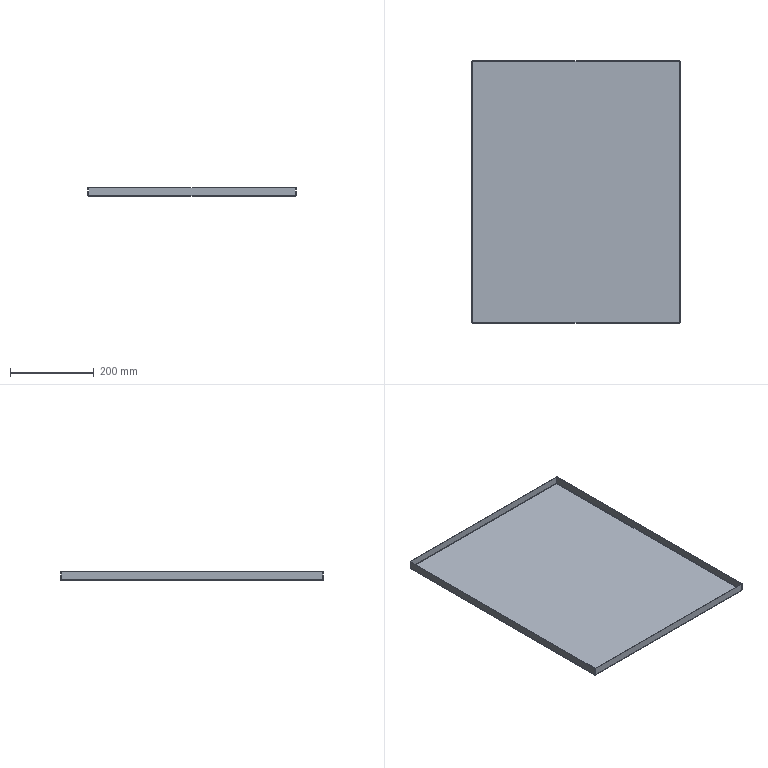Part | STEP file | X77-03024 | 1 solid | 38 faces | box 498 x 628 x 20 mm | volume 528951 mm3 | plane 22 | spline 8 | cylinder 8 | commonest cylinder face diameters 1.473 x4 4.473 x4